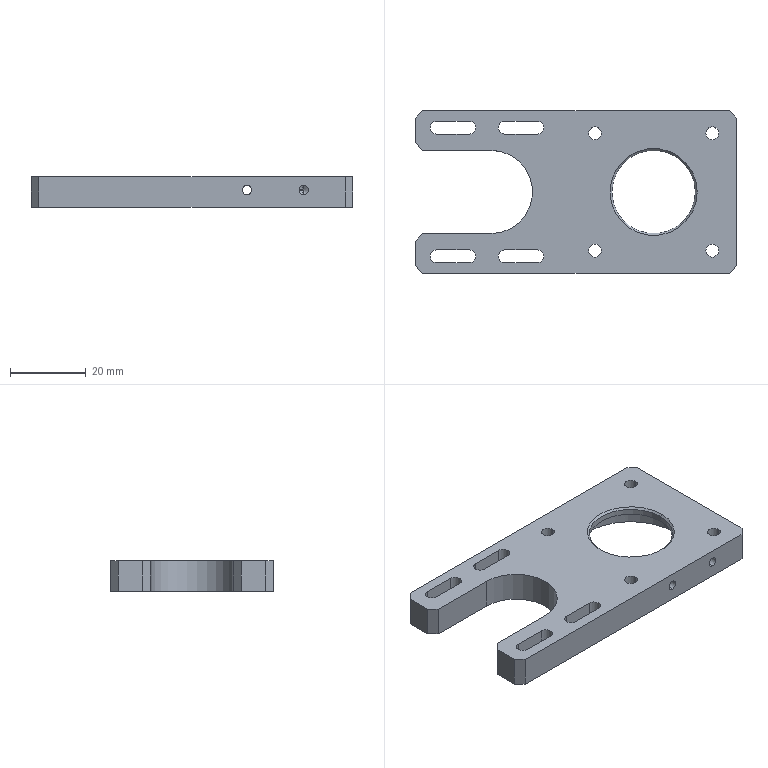Part | NX | features BREP 1 | 1 solid | 99 faces | box 85 x 43 x 8 mm | volume 15446 mm3 | cylinder 53 | plane 40 | cone 6 | commonest cylinder face diameters 3.4 x20 7.2 x12 2.5 x8 7 x8 22 x3 32 x2